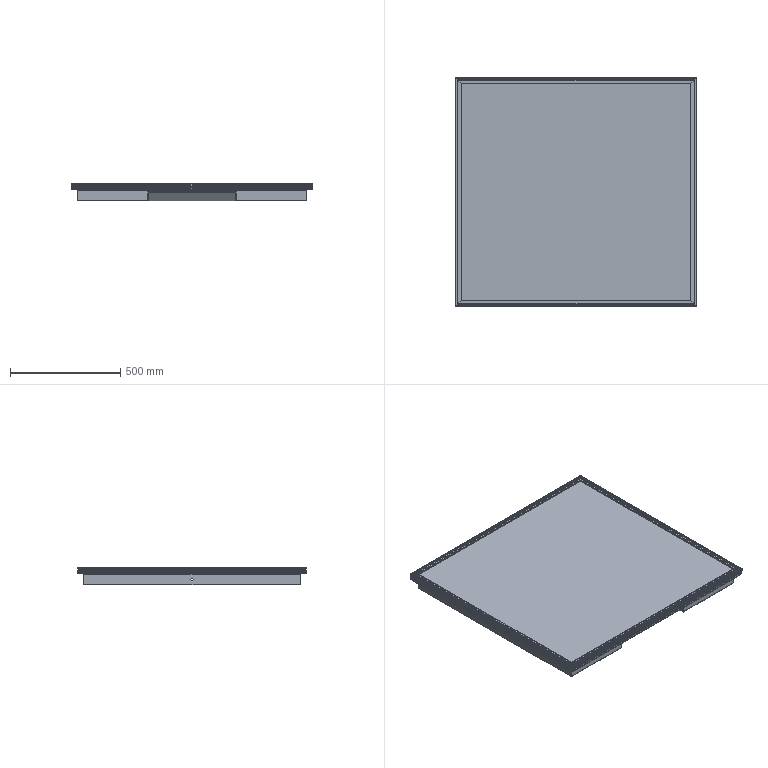Part | 7 solids | 486 faces | box 1095 x 1035 x 80.189 mm | volume 25091313 mm3 | plane 332 | cylinder 142 | spline 12 | commonest cylinder face diameters 7 x50 0.4 x37 2 x16 11 x14 2.4 x11 1 x8